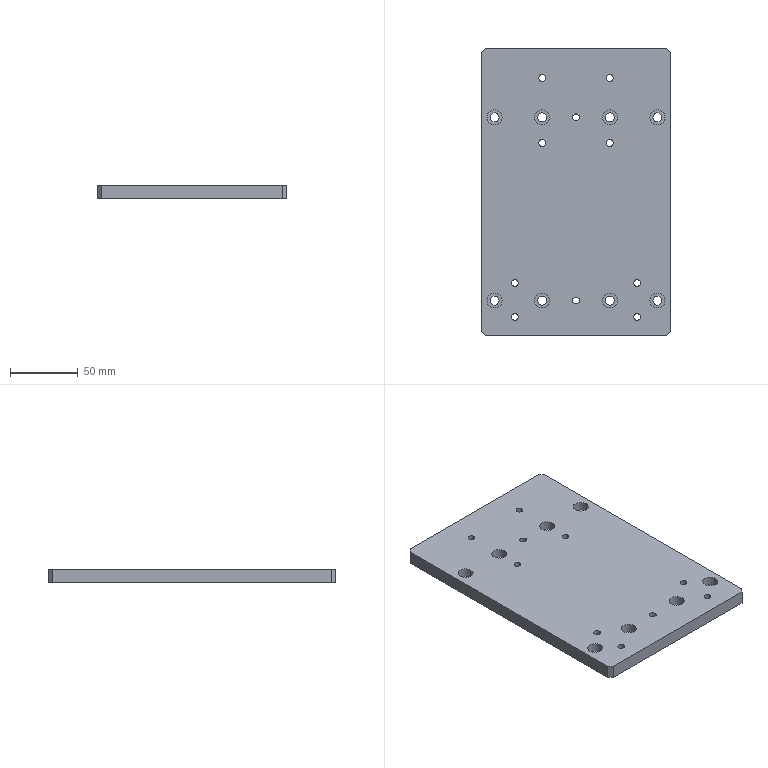Part | NX | features BREP 1 | 1 solid | 70 faces | box 140 x 212 x 10 mm | volume 288611 mm3 | cylinder 52 | plane 18 | commonest cylinder face diameters 5 x20 6.6 x16 11 x16